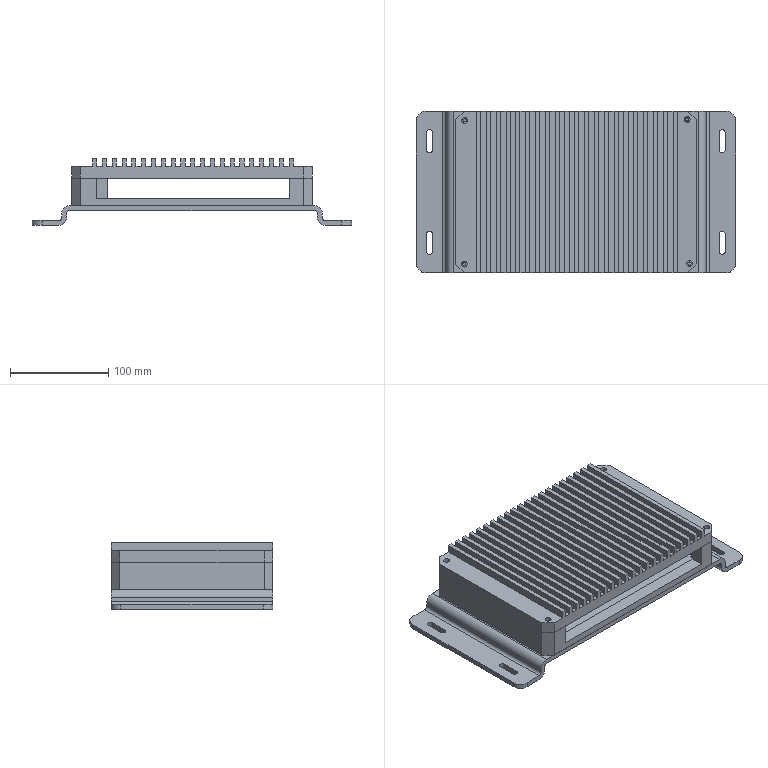Part | NX | features BREP 3 | 3 solids | 202 faces | box 325.101 x 164.735 x 67.855 mm | volume 1193658 mm3 | plane 162 | cylinder 40 | commonest cylinder face diameters 6 x16 3.2 x8 3 x4 6.5 x4 16 x4 20 x4